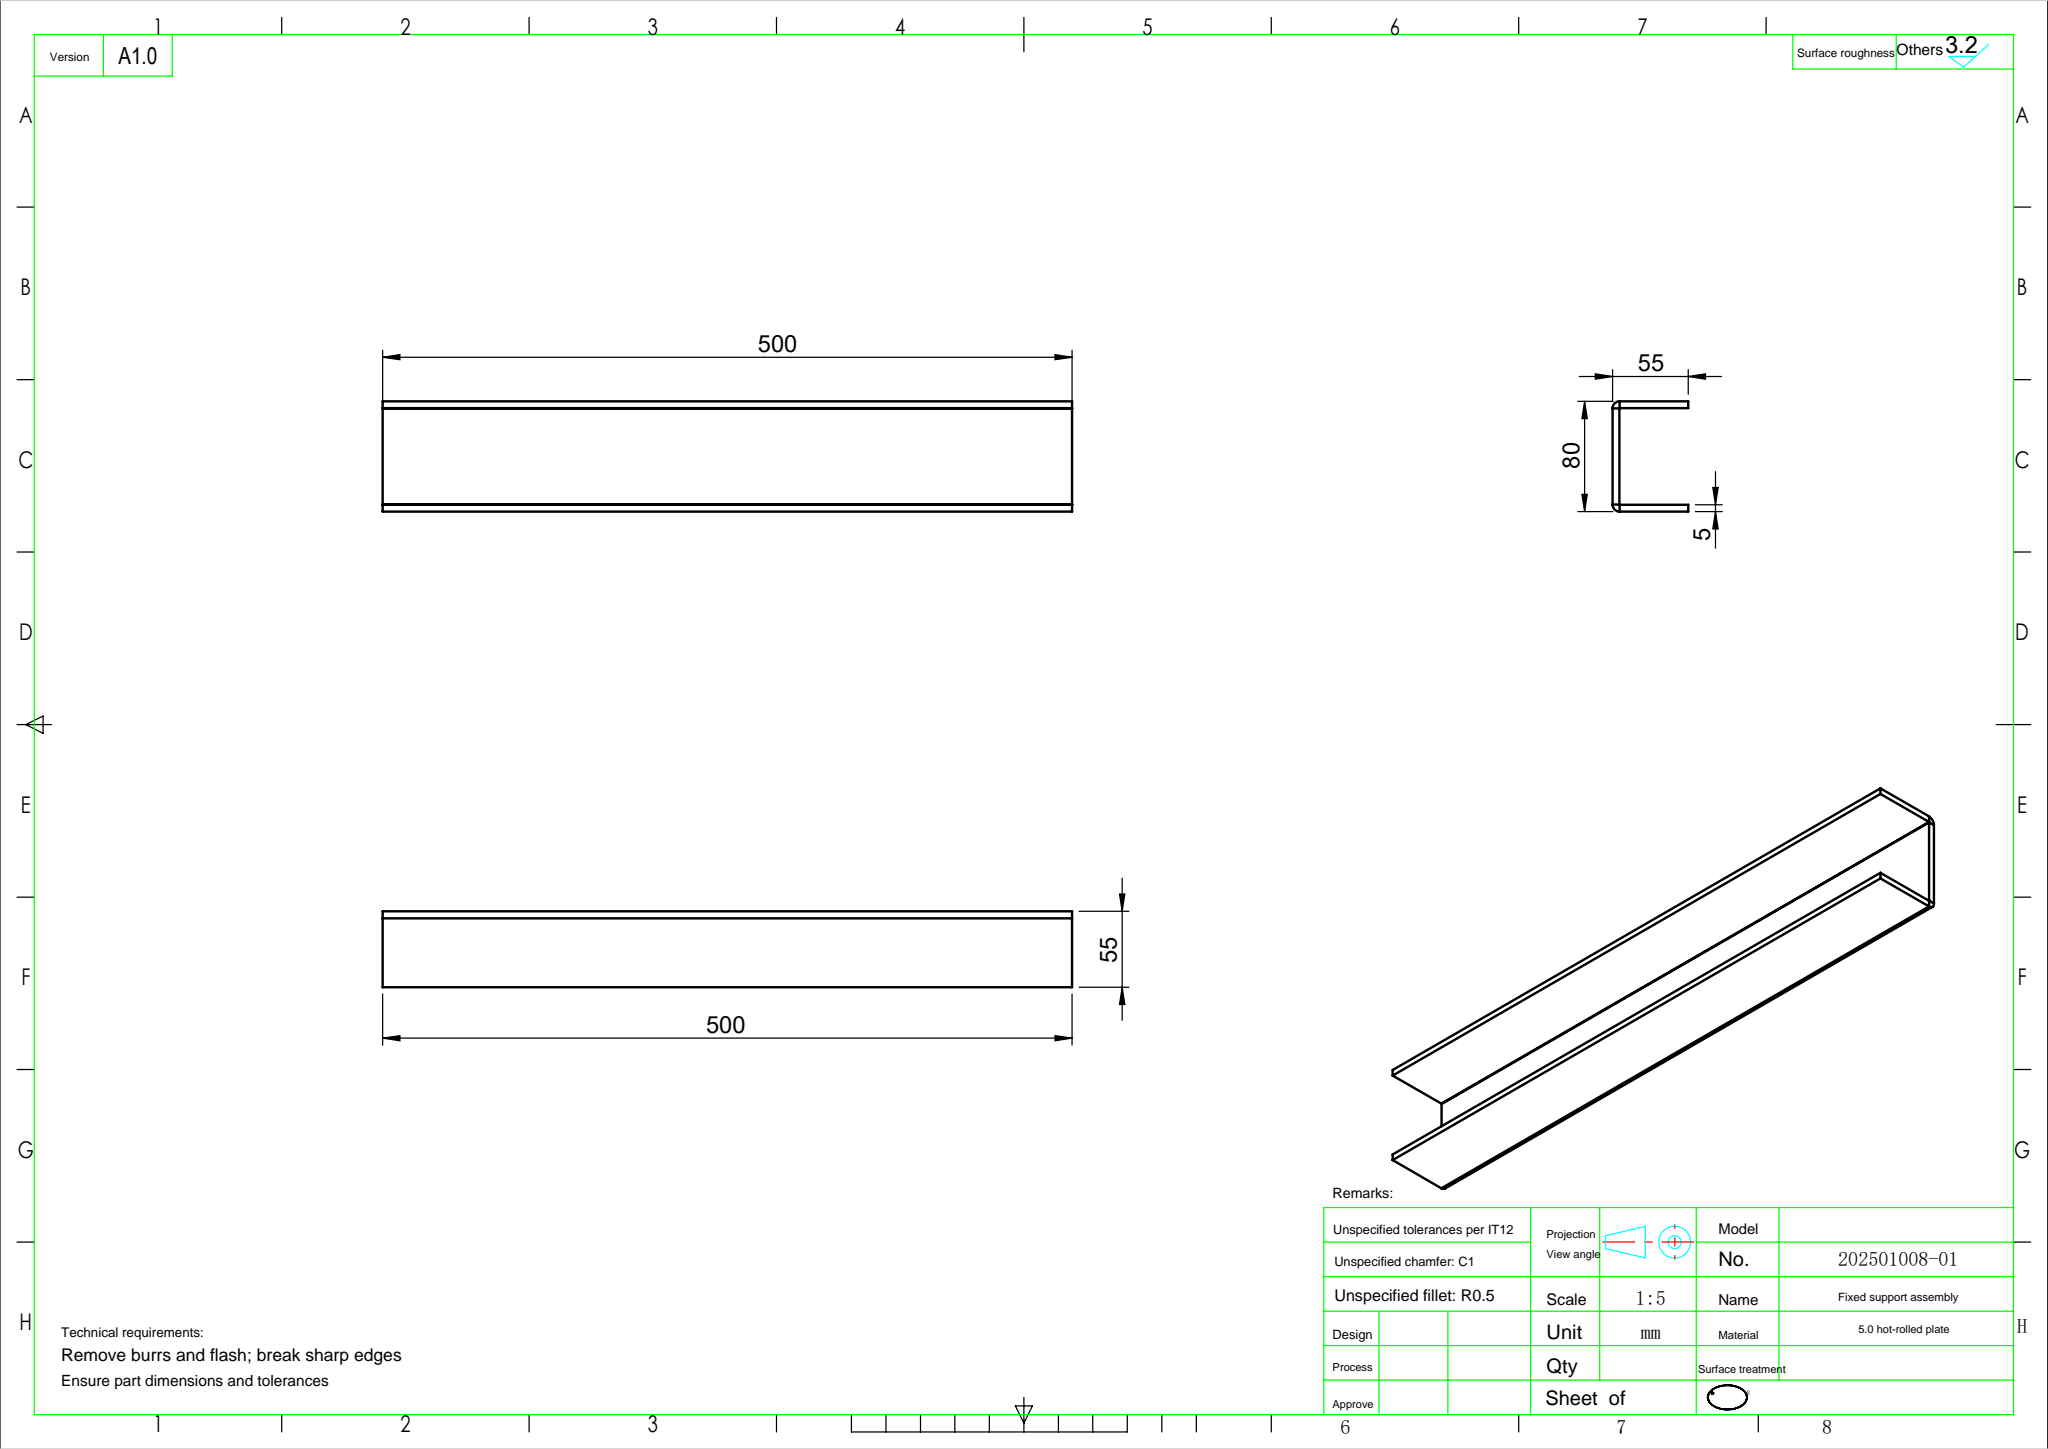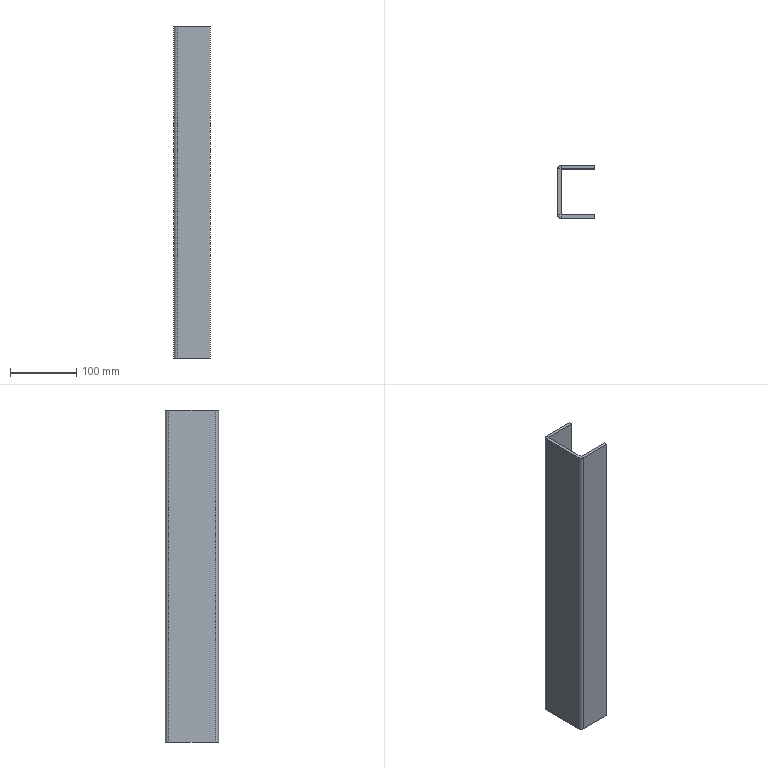Part | SolidWorks | features FlatPattern 1, SMBaseFlange 1, SheetMetal 1 | 1 solid | 22 faces | box 55 x 80 x 500 mm | volume 444206 mm3 | plane 18 | cylinder 4 | commonest cylinder face diameters 0.4 x2 10.4 x2
STEP:
#1=CARTESIAN_POINT('',(0.,34.8,500.));
#2=VERTEX_POINT('',#1);
#3=CARTESIAN_POINT('',(-5.,34.8,500.));
#4=VERTEX_POINT('',#3);
#5=CARTESIAN_POINT('',(0.,34.8,500.));
#6=DIRECTION('',(-1.,0.,0.));
#7=VECTOR('',#6,1000.);
#8=LINE('',#5,#7);
#9=EDGE_CURVE('',#2,#4,#8,.T.);
#10=ORIENTED_EDGE('',*,*,#9,.F.);
#11=CARTESIAN_POINT('',(0.2,35.,500.));
#12=VERTEX_POINT('',#11);
#13=CARTESIAN_POINT('',(0.2,34.8,500.));
#14=DIRECTION('',(0.,0.,1.));
#15=DIRECTION('',(-1.,0.,0.));
#16=AXIS2_PLACEMENT_3D('',#13,#14,#15);
#17=CIRCLE('',#16,0.2);
#18=EDGE_CURVE('',#12,#2,#17,.T.);
#19=ORIENTED_EDGE('',*,*,#18,.F.);
#20=CARTESIAN_POINT('',(0.2,40.,500.));
#21=VERTEX_POINT('',#20);
#22=CARTESIAN_POINT('',(0.2,40.,500.));
#23=DIRECTION('',(0.,-1.,0.));
#24=VECTOR('',#23,1000.);
#25=LINE('',#22,#24);
#26=EDGE_CURVE('',#21,#12,#25,.T.);
#27=ORIENTED_EDGE('',*,*,#26,.F.);
#28=CARTESIAN_POINT('',(0.2,34.8,500.));
#29=DIRECTION('',(0.,0.,1.));
#30=DIRECTION('',(1.,0.,0.));
#31=AXIS2_PLACEMENT_3D('',#28,#29,#30);
#32=CIRCLE('',#31,5.2);
#33=EDGE_CURVE('',#21,#4,#32,.T.);
#34=ORIENTED_EDGE('',*,*,#33,.T.);
#35=EDGE_LOOP('',(#10,#19,#27,#34));
#36=FACE_OUTER_BOUND('',#35,.T.);
#37=CARTESIAN_POINT('',(0.,34.8,500.));
#38=DIRECTION('',(0.,0.,1.));
#39=DIRECTION('',(1.,0.,0.));
#40=AXIS2_PLACEMENT_3D('',#37,#38,#39);
#41=PLANE('',#40);
#42=ADVANCED_FACE('',(#36),#41,.T.);
#43=CARTESIAN_POINT('',(0.,-34.8,500.));
#44=VERTEX_POINT('',#43);
#45=CARTESIAN_POINT('',(0.,35.,500.));
#46=DIRECTION('',(0.,-1.,0.));
#47=VECTOR('',#46,1000.);
#48=LINE('',#45,#47);
#49=EDGE_CURVE('',#2,#44,#48,.T.);
#50=ORIENTED_EDGE('',*,*,#49,.F.);
#51=ORIENTED_EDGE('',*,*,#9,.T.);
#52=CARTESIAN_POINT('',(-5.,-34.8,500.));
#53=VERTEX_POINT('',#52);
#54=CARTESIAN_POINT('',(-5.,35.,500.));
#55=DIRECTION('',(0.,-1.,0.));
#56=VECTOR('',#55,1000.);
#57=LINE('',#54,#56);
#58=EDGE_CURVE('',#4,#53,#57,.T.);
#59=ORIENTED_EDGE('',*,*,#58,.T.);
#60=CARTESIAN_POINT('',(-5.,-34.8,500.));
#61=DIRECTION('',(1.,0.,0.));
#62=VECTOR('',#61,1000.);
#63=LINE('',#60,#62);
#64=EDGE_CURVE('',#53,#44,#63,.T.);
#65=ORIENTED_EDGE('',*,*,#64,.T.);
#66=EDGE_LOOP('',(#50,#51,#59,#65));
#67=FACE_OUTER_BOUND('',#66,.T.);
#68=CARTESIAN_POINT('',(0.2,40.,500.));
#69=DIRECTION('',(0.,0.,1.));
#70=DIRECTION('',(1.,0.,0.));
#71=AXIS2_PLACEMENT_3D('',#68,#69,#70);
#72=PLANE('',#71);
#73=ADVANCED_FACE('',(#67),#72,.T.);
#74=CARTESIAN_POINT('',(0.2,35.,0.));
#75=VERTEX_POINT('',#74);
#76=CARTESIAN_POINT('',(0.2,40.,0.));
#77=VERTEX_POINT('',#76);
#78=CARTESIAN_POINT('',(0.2,35.,0.));
#79=DIRECTION('',(0.,1.,0.));
#80=VECTOR('',#79,1000.);
#81=LINE('',#78,#80);
#82=EDGE_CURVE('',#75,#77,#81,.T.);
#83=ORIENTED_EDGE('',*,*,#82,.F.);
#84=CARTESIAN_POINT('',(0.,34.8,0.));
#85=VERTEX_POINT('',#84);
#86=CARTESIAN_POINT('',(0.2,34.8,0.));
#87=DIRECTION('',(0.,0.,1.));
#88=DIRECTION('',(-1.,0.,0.));
#89=AXIS2_PLACEMENT_3D('',#86,#87,#88);
#90=CIRCLE('',#89,0.2);
#91=EDGE_CURVE('',#75,#85,#90,.T.);
#92=ORIENTED_EDGE('',*,*,#91,.T.);
#93=CARTESIAN_POINT('',(-5.,34.8,0.));
#94=VERTEX_POINT('',#93);
#95=CARTESIAN_POINT('',(-5.,34.8,0.));
#96=DIRECTION('',(1.,0.,0.));
#97=VECTOR('',#96,1000.);
#98=LINE('',#95,#97);
#99=EDGE_CURVE('',#94,#85,#98,.T.);
#100=ORIENTED_EDGE('',*,*,#99,.F.);
#101=CARTESIAN_POINT('',(0.2,34.8,0.));
#102=DIRECTION('',(0.,0.,1.));
#103=DIRECTION('',(1.,0.,0.));
#104=AXIS2_PLACEMENT_3D('',#101,#102,#103);
#105=CIRCLE('',#104,5.2);
#106=EDGE_CURVE('',#77,#94,#105,.T.);
#107=ORIENTED_EDGE('',*,*,#106,.F.);
#108=EDGE_LOOP('',(#83,#92,#100,#107));
#109=FACE_OUTER_BOUND('',#108,.T.);
#110=CARTESIAN_POINT('',(0.2,35.,0.));
#111=DIRECTION('',(0.,0.,-1.));
#112=DIRECTION('',(-1.,0.,0.));
#113=AXIS2_PLACEMENT_3D('',#110,#111,#112);
#114=PLANE('',#113);
#115=ADVANCED_FACE('',(#109),#114,.T.);
#116=CARTESIAN_POINT('',(50.,35.,0.));
#117=VERTEX_POINT('',#116);
#118=CARTESIAN_POINT('',(0.,35.,0.));
#119=DIRECTION('',(-1.,0.,0.));
#120=VECTOR('',#119,1000.);
#121=LINE('',#118,#120);
#122=EDGE_CURVE('',#117,#75,#121,.T.);
#123=ORIENTED_EDGE('',*,*,#122,.T.);
#124=ORIENTED_EDGE('',*,*,#82,.T.);
#125=CARTESIAN_POINT('',(50.,40.,0.));
#126=VERTEX_POINT('',#125);
#127=CARTESIAN_POINT('',(0.,40.,0.));
#128=DIRECTION('',(-1.,0.,0.));
#129=VECTOR('',#128,1000.);
#130=LINE('',#127,#129);
#131=EDGE_CURVE('',#126,#77,#130,.T.);
#132=ORIENTED_EDGE('',*,*,#131,.F.);
#133=CARTESIAN_POINT('',(50.,40.,0.));
#134=DIRECTION('',(0.,-1.,0.));
#135=VECTOR('',#134,1000.);
#136=LINE('',#133,#135);
#137=EDGE_CURVE('',#126,#117,#136,.T.);
#138=ORIENTED_EDGE('',*,*,#137,.T.);
#139=EDGE_LOOP('',(#123,#124,#132,#138));
#140=FACE_OUTER_BOUND('',#139,.T.);
#141=CARTESIAN_POINT('',(-5.,34.8,0.));
#142=DIRECTION('',(0.,0.,-1.));
#143=DIRECTION('',(-1.,0.,0.));
#144=AXIS2_PLACEMENT_3D('',#141,#142,#143);
#145=PLANE('',#144);
#146=ADVANCED_FACE('',(#140),#145,.T.);
#147=CARTESIAN_POINT('',(0.2,-35.,500.));
#148=VERTEX_POINT('',#147);
#149=CARTESIAN_POINT('',(0.2,-40.,500.));
#150=VERTEX_POINT('',#149);
#151=CARTESIAN_POINT('',(0.2,-35.,500.));
#152=DIRECTION('',(0.,-1.,0.));
#153=VECTOR('',#152,1000.);
#154=LINE('',#151,#153);
#155=EDGE_CURVE('',#148,#150,#154,.T.);
#156=ORIENTED_EDGE('',*,*,#155,.F.);
#157=CARTESIAN_POINT('',(0.2,-34.8,500.));
#158=DIRECTION('',(0.,0.,1.));
#159=DIRECTION('',(-1.,0.,0.));
#160=AXIS2_PLACEMENT_3D('',#157,#158,#159);
#161=CIRCLE('',#160,0.2);
#162=EDGE_CURVE('',#44,#148,#161,.T.);
#163=ORIENTED_EDGE('',*,*,#162,.F.);
#164=ORIENTED_EDGE('',*,*,#64,.F.);
#165=CARTESIAN_POINT('',(0.2,-34.8,500.));
#166=DIRECTION('',(0.,0.,1.));
#167=DIRECTION('',(1.,0.,0.));
#168=AXIS2_PLACEMENT_3D('',#165,#166,#167);
#169=CIRCLE('',#168,5.2);
#170=EDGE_CURVE('',#53,#150,#169,.T.);
#171=ORIENTED_EDGE('',*,*,#170,.T.);
#172=EDGE_LOOP('',(#156,#163,#164,#171));
#173=FACE_OUTER_BOUND('',#172,.T.);
#174=CARTESIAN_POINT('',(0.2,-35.,500.));
#175=DIRECTION('',(0.,0.,1.));
#176=DIRECTION('',(1.,0.,0.));
#177=AXIS2_PLACEMENT_3D('',#174,#175,#176);
#178=PLANE('',#177);
#179=ADVANCED_FACE('',(#173),#178,.T.);
#180=CARTESIAN_POINT('',(50.,-35.,500.));
#181=VERTEX_POINT('',#180);
#182=CARTESIAN_POINT('',(0.,-35.,500.));
#183=DIRECTION('',(1.,0.,0.));
#184=VECTOR('',#183,1000.);
#185=LINE('',#182,#184);
#186=EDGE_CURVE('',#148,#181,#185,.T.);
#187=ORIENTED_EDGE('',*,*,#186,.F.);
#188=ORIENTED_EDGE('',*,*,#155,.T.);
#189=CARTESIAN_POINT('',(50.,-40.,500.));
#190=VERTEX_POINT('',#189);
#191=CARTESIAN_POINT('',(0.,-40.,500.));
#192=DIRECTION('',(1.,0.,0.));
#193=VECTOR('',#192,1000.);
#194=LINE('',#191,#193);
#195=EDGE_CURVE('',#150,#190,#194,.T.);
#196=ORIENTED_EDGE('',*,*,#195,.T.);
#197=CARTESIAN_POINT('',(50.,-35.,500.));
#198=DIRECTION('',(0.,-1.,0.));
#199=VECTOR('',#198,1000.);
#200=LINE('',#197,#199);
#201=EDGE_CURVE('',#181,#190,#200,.T.);
#202=ORIENTED_EDGE('',*,*,#201,.F.);
#203=EDGE_LOOP('',(#187,#188,#196,#202));
#204=FACE_OUTER_BOUND('',#203,.T.);
#205=CARTESIAN_POINT('',(-5.,-34.8,500.));
#206=DIRECTION('',(0.,0.,1.));
#207=DIRECTION('',(1.,0.,0.));
#208=AXIS2_PLACEMENT_3D('',#205,#206,#207);
#209=PLANE('',#208);
#210=ADVANCED_FACE('',(#204),#209,.T.);
#211=CARTESIAN_POINT('',(0.,-34.8,0.));
#212=VERTEX_POINT('',#211);
#213=CARTESIAN_POINT('',(-5.,-34.8,0.));
#214=VERTEX_POINT('',#213);
#215=CARTESIAN_POINT('',(0.,-34.8,0.));
#216=DIRECTION('',(-1.,0.,0.));
#217=VECTOR('',#216,1000.);
#218=LINE('',#215,#217);
#219=EDGE_CURVE('',#212,#214,#218,.T.);
#220=ORIENTED_EDGE('',*,*,#219,.F.);
#221=CARTESIAN_POINT('',(0.2,-35.,0.));
#222=VERTEX_POINT('',#221);
#223=CARTESIAN_POINT('',(0.2,-34.8,0.));
#224=DIRECTION('',(0.,0.,1.));
#225=DIRECTION('',(-1.,0.,0.));
#226=AXIS2_PLACEMENT_3D('',#223,#224,#225);
#227=CIRCLE('',#226,0.2);
#228=EDGE_CURVE('',#212,#222,#227,.T.);
#229=ORIENTED_EDGE('',*,*,#228,.T.);
#230=CARTESIAN_POINT('',(0.2,-40.,0.));
#231=VERTEX_POINT('',#230);
#232=CARTESIAN_POINT('',(0.2,-40.,0.));
#233=DIRECTION('',(0.,1.,0.));
#234=VECTOR('',#233,1000.);
#235=LINE('',#232,#234);
#236=EDGE_CURVE('',#231,#222,#235,.T.);
#237=ORIENTED_EDGE('',*,*,#236,.F.);
#238=CARTESIAN_POINT('',(0.2,-34.8,0.));
#239=DIRECTION('',(0.,0.,1.));
#240=DIRECTION('',(1.,0.,0.));
#241=AXIS2_PLACEMENT_3D('',#238,#239,#240);
#242=CIRCLE('',#241,5.2);
#243=EDGE_CURVE('',#214,#231,#242,.T.);
#244=ORIENTED_EDGE('',*,*,#243,.F.);
#245=EDGE_LOOP('',(#220,#229,#237,#244));
#246=FACE_OUTER_BOUND('',#245,.T.);
#247=CARTESIAN_POINT('',(0.,-34.8,0.));
#248=DIRECTION('',(0.,0.,-1.));
#249=DIRECTION('',(-1.,0.,0.));
#250=AXIS2_PLACEMENT_3D('',#247,#248,#249);
#251=PLANE('',#250);
#252=ADVANCED_FACE('',(#246),#251,.T.);
#253=CARTESIAN_POINT('',(0.,35.,0.));
#254=DIRECTION('',(0.,-1.,0.));
#255=VECTOR('',#254,1000.);
#256=LINE('',#253,#255);
#257=EDGE_CURVE('',#85,#212,#256,.T.);
#258=ORIENTED_EDGE('',*,*,#257,.T.);
#259=ORIENTED_EDGE('',*,*,#219,.T.);
#260=CARTESIAN_POINT('',(-5.,35.,0.));
#261=DIRECTION('',(0.,-1.,0.));
#262=VECTOR('',#261,1000.);
#263=LINE('',#260,#262);
#264=EDGE_CURVE('',#94,#214,#263,.T.);
#265=ORIENTED_EDGE('',*,*,#264,.F.);
#266=ORIENTED_EDGE('',*,*,#99,.T.);
#267=EDGE_LOOP('',(#258,#259,#265,#266));
#268=FACE_OUTER_BOUND('',#267,.T.);
#269=CARTESIAN_POINT('',(0.2,-40.,0.));
#270=DIRECTION('',(0.,0.,-1.));
#271=DIRECTION('',(-1.,0.,0.));
#272=AXIS2_PLACEMENT_3D('',#269,#270,#271);
#273=PLANE('',#272);
#274=ADVANCED_FACE('',(#268),#273,.T.);
#275=CARTESIAN_POINT('',(50.,-40.,0.));
#276=VERTEX_POINT('',#275);
#277=CARTESIAN_POINT('',(0.,-40.,0.));
#278=DIRECTION('',(1.,0.,0.));
#279=VECTOR('',#278,1000.);
#280=LINE('',#277,#279);
#281=EDGE_CURVE('',#231,#276,#280,.T.);
#282=ORIENTED_EDGE('',*,*,#281,.T.);
#283=CARTESIAN_POINT('',(50.,-40.,500.));
#284=DIRECTION('',(0.,0.,-1.));
#285=VECTOR('',#284,1000.);
#286=LINE('',#283,#285);
#287=EDGE_CURVE('',#190,#276,#286,.T.);
#288=ORIENTED_EDGE('',*,*,#287,.F.);
#289=ORIENTED_EDGE('',*,*,#195,.F.);
#290=CARTESIAN_POINT('',(0.2,-40.,500.));
#291=DIRECTION('',(0.,0.,-1.));
#292=VECTOR('',#291,1000.);
#293=LINE('',#290,#292);
#294=EDGE_CURVE('',#150,#231,#293,.T.);
#295=ORIENTED_EDGE('',*,*,#294,.T.);
#296=EDGE_LOOP('',(#282,#288,#289,#295));
#297=FACE_OUTER_BOUND('',#296,.T.);
#298=CARTESIAN_POINT('',(0.,-40.,500.));
#299=DIRECTION('',(0.,1.,0.));
#300=DIRECTION('',(0.,0.,1.));
#301=AXIS2_PLACEMENT_3D('',#298,#299,#300);
#302=PLANE('',#301);
#303=ADVANCED_FACE('',(#297),#302,.F.);
#304=CARTESIAN_POINT('',(50.,-35.,0.));
#305=VERTEX_POINT('',#304);
#306=CARTESIAN_POINT('',(50.,-35.,0.));
#307=DIRECTION('',(0.,-1.,0.));
#308=VECTOR('',#307,1000.);
#309=LINE('',#306,#308);
#310=EDGE_CURVE('',#305,#276,#309,.T.);
#311=ORIENTED_EDGE('',*,*,#310,.F.);
#312=CARTESIAN_POINT('',(50.,-35.,500.));
#313=DIRECTION('',(0.,0.,-1.));
#314=VECTOR('',#313,1000.);
#315=LINE('',#312,#314);
#316=EDGE_CURVE('',#181,#305,#315,.T.);
#317=ORIENTED_EDGE('',*,*,#316,.F.);
#318=ORIENTED_EDGE('',*,*,#201,.T.);
#319=ORIENTED_EDGE('',*,*,#287,.T.);
#320=EDGE_LOOP('',(#311,#317,#318,#319));
#321=FACE_OUTER_BOUND('',#320,.T.);
#322=CARTESIAN_POINT('',(50.,-35.,500.));
#323=DIRECTION('',(1.,0.,0.));
#324=DIRECTION('',(0.,0.,-1.));
#325=AXIS2_PLACEMENT_3D('',#322,#323,#324);
#326=PLANE('',#325);
#327=ADVANCED_FACE('',(#321),#326,.T.);
#328=CARTESIAN_POINT('',(0.,-35.,0.));
#329=DIRECTION('',(1.,0.,0.));
#330=VECTOR('',#329,1000.);
#331=LINE('',#328,#330);
#332=EDGE_CURVE('',#222,#305,#331,.T.);
#333=ORIENTED_EDGE('',*,*,#332,.F.);
#334=CARTESIAN_POINT('',(0.2,-35.,500.));
#335=DIRECTION('',(0.,0.,-1.));
#336=VECTOR('',#335,1000.);
#337=LINE('',#334,#336);
#338=EDGE_CURVE('',#148,#222,#337,.T.);
#339=ORIENTED_EDGE('',*,*,#338,.F.);
#340=ORIENTED_EDGE('',*,*,#186,.T.);
#341=ORIENTED_EDGE('',*,*,#316,.T.);
#342=EDGE_LOOP('',(#333,#339,#340,#341));
#343=FACE_OUTER_BOUND('',#342,.T.);
#344=CARTESIAN_POINT('',(0.,-35.,500.));
#345=DIRECTION('',(0.,1.,0.));
#346=DIRECTION('',(0.,0.,1.));
#347=AXIS2_PLACEMENT_3D('',#344,#345,#346);
#348=PLANE('',#347);
#349=ADVANCED_FACE('',(#343),#348,.T.);
#350=ORIENTED_EDGE('',*,*,#228,.F.);
#351=CARTESIAN_POINT('',(0.,-34.8,500.));
#352=DIRECTION('',(0.,0.,-1.));
#353=VECTOR('',#352,1000.);
#354=LINE('',#351,#353);
#355=EDGE_CURVE('',#44,#212,#354,.T.);
#356=ORIENTED_EDGE('',*,*,#355,.F.);
#357=ORIENTED_EDGE('',*,*,#162,.T.);
#358=ORIENTED_EDGE('',*,*,#338,.T.);
#359=EDGE_LOOP('',(#350,#356,#357,#358));
#360=FACE_OUTER_BOUND('',#359,.T.);
#361=CARTESIAN_POINT('',(0.2,-34.8,500.));
#362=DIRECTION('',(0.,0.,-1.));
#363=DIRECTION('',(-1.,0.,0.));
#364=AXIS2_PLACEMENT_3D('',#361,#362,#363);
#365=CYLINDRICAL_SURFACE('',#364,0.2);
#366=ADVANCED_FACE('',(#360),#365,.F.);
#367=ORIENTED_EDGE('',*,*,#257,.F.);
#368=CARTESIAN_POINT('',(0.,34.8,500.));
#369=DIRECTION('',(0.,0.,-1.));
#370=VECTOR('',#369,1000.);
#371=LINE('',#368,#370);
#372=EDGE_CURVE('',#2,#85,#371,.T.);
#373=ORIENTED_EDGE('',*,*,#372,.F.);
#374=ORIENTED_EDGE('',*,*,#49,.T.);
#375=ORIENTED_EDGE('',*,*,#355,.T.);
#376=EDGE_LOOP('',(#367,#373,#374,#375));
#377=FACE_OUTER_BOUND('',#376,.T.);
#378=CARTESIAN_POINT('',(0.,35.,500.));
#379=DIRECTION('',(1.,0.,0.));
#380=DIRECTION('',(0.,0.,-1.));
#381=AXIS2_PLACEMENT_3D('',#378,#379,#380);
#382=PLANE('',#381);
#383=ADVANCED_FACE('',(#377),#382,.T.);
#384=ORIENTED_EDGE('',*,*,#91,.F.);
#385=CARTESIAN_POINT('',(0.2,35.,500.));
#386=DIRECTION('',(0.,0.,-1.));
#387=VECTOR('',#386,1000.);
#388=LINE('',#385,#387);
#389=EDGE_CURVE('',#12,#75,#388,.T.);
#390=ORIENTED_EDGE('',*,*,#389,.F.);
#391=ORIENTED_EDGE('',*,*,#18,.T.);
#392=ORIENTED_EDGE('',*,*,#372,.T.);
#393=EDGE_LOOP('',(#384,#390,#391,#392));
#394=FACE_OUTER_BOUND('',#393,.T.);
#395=CARTESIAN_POINT('',(0.2,34.8,500.));
#396=DIRECTION('',(0.,0.,-1.));
#397=DIRECTION('',(-1.,0.,0.));
#398=AXIS2_PLACEMENT_3D('',#395,#396,#397);
#399=CYLINDRICAL_SURFACE('',#398,0.2);
#400=ADVANCED_FACE('',(#394),#399,.F.);
#401=ORIENTED_EDGE('',*,*,#122,.F.);
#402=CARTESIAN_POINT('',(50.,35.,500.));
#403=VERTEX_POINT('',#402);
#404=CARTESIAN_POINT('',(50.,35.,500.));
#405=DIRECTION('',(0.,0.,-1.));
#406=VECTOR('',#405,1000.);
#407=LINE('',#404,#406);
#408=EDGE_CURVE('',#403,#117,#407,.T.);
#409=ORIENTED_EDGE('',*,*,#408,.F.);
#410=CARTESIAN_POINT('',(0.,35.,500.));
#411=DIRECTION('',(-1.,0.,0.));
#412=VECTOR('',#411,1000.);
#413=LINE('',#410,#412);
#414=EDGE_CURVE('',#403,#12,#413,.T.);
#415=ORIENTED_EDGE('',*,*,#414,.T.);
#416=ORIENTED_EDGE('',*,*,#389,.T.);
#417=EDGE_LOOP('',(#401,#409,#415,#416));
#418=FACE_OUTER_BOUND('',#417,.T.);
#419=CARTESIAN_POINT('',(0.,35.,500.));
#420=DIRECTION('',(0.,-1.,0.));
#421=DIRECTION('',(0.,0.,-1.));
#422=AXIS2_PLACEMENT_3D('',#419,#420,#421);
#423=PLANE('',#422);
#424=ADVANCED_FACE('',(#418),#423,.T.);
#425=ORIENTED_EDGE('',*,*,#137,.F.);
#426=CARTESIAN_POINT('',(50.,40.,500.));
#427=VERTEX_POINT('',#426);
#428=CARTESIAN_POINT('',(50.,40.,500.));
#429=DIRECTION('',(0.,0.,-1.));
#430=VECTOR('',#429,1000.);
#431=LINE('',#428,#430);
#432=EDGE_CURVE('',#427,#126,#431,.T.);
#433=ORIENTED_EDGE('',*,*,#432,.F.);
#434=CARTESIAN_POINT('',(50.,40.,500.));
#435=DIRECTION('',(0.,-1.,0.));
#436=VECTOR('',#435,1000.);
#437=LINE('',#434,#436);
#438=EDGE_CURVE('',#427,#403,#437,.T.);
#439=ORIENTED_EDGE('',*,*,#438,.T.);
#440=ORIENTED_EDGE('',*,*,#408,.T.);
#441=EDGE_LOOP('',(#425,#433,#439,#440));
#442=FACE_OUTER_BOUND('',#441,.T.);
#443=CARTESIAN_POINT('',(50.,40.,500.));
#444=DIRECTION('',(1.,0.,0.));
#445=DIRECTION('',(0.,0.,-1.));
#446=AXIS2_PLACEMENT_3D('',#443,#444,#445);
#447=PLANE('',#446);
#448=ADVANCED_FACE('',(#442),#447,.T.);
#449=ORIENTED_EDGE('',*,*,#131,.T.);
#450=CARTESIAN_POINT('',(0.2,40.,500.));
#451=DIRECTION('',(0.,0.,-1.));
#452=VECTOR('',#451,1000.);
#453=LINE('',#450,#452);
#454=EDGE_CURVE('',#21,#77,#453,.T.);
#455=ORIENTED_EDGE('',*,*,#454,.F.);
#456=CARTESIAN_POINT('',(0.,40.,500.));
#457=DIRECTION('',(-1.,0.,0.));
#458=VECTOR('',#457,1000.);
#459=LINE('',#456,#458);
#460=EDGE_CURVE('',#427,#21,#459,.T.);
#461=ORIENTED_EDGE('',*,*,#460,.F.);
#462=ORIENTED_EDGE('',*,*,#432,.T.);
#463=EDGE_LOOP('',(#449,#455,#461,#462));
#464=FACE_OUTER_BOUND('',#463,.T.);
#465=CARTESIAN_POINT('',(0.,40.,500.));
#466=DIRECTION('',(0.,-1.,0.));
#467=DIRECTION('',(0.,0.,-1.));
#468=AXIS2_PLACEMENT_3D('',#465,#466,#467);
#469=PLANE('',#468);
#470=ADVANCED_FACE('',(#464),#469,.F.);
#471=ORIENTED_EDGE('',*,*,#106,.T.);
#472=CARTESIAN_POINT('',(-5.,34.8,500.));
#473=DIRECTION('',(0.,0.,-1.));
#474=VECTOR('',#473,1000.);
#475=LINE('',#472,#474);
#476=EDGE_CURVE('',#4,#94,#475,.T.);
#477=ORIENTED_EDGE('',*,*,#476,.F.);
#478=ORIENTED_EDGE('',*,*,#33,.F.);
#479=ORIENTED_EDGE('',*,*,#454,.T.);
#480=EDGE_LOOP('',(#471,#477,#478,#479));
#481=FACE_OUTER_BOUND('',#480,.T.);
#482=CARTESIAN_POINT('',(0.2,34.8,500.));
#483=DIRECTION('',(0.,0.,-1.));
#484=DIRECTION('',(-1.,0.,0.));
#485=AXIS2_PLACEMENT_3D('',#482,#483,#484);
#486=CYLINDRICAL_SURFACE('',#485,5.2);
#487=ADVANCED_FACE('',(#481),#486,.T.);
#488=ORIENTED_EDGE('',*,*,#264,.T.);
#489=CARTESIAN_POINT('',(-5.,-34.8,500.));
#490=DIRECTION('',(0.,0.,-1.));
#491=VECTOR('',#490,1000.);
#492=LINE('',#489,#491);
#493=EDGE_CURVE('',#53,#214,#492,.T.);
#494=ORIENTED_EDGE('',*,*,#493,.F.);
#495=ORIENTED_EDGE('',*,*,#58,.F.);
#496=ORIENTED_EDGE('',*,*,#476,.T.);
#497=EDGE_LOOP('',(#488,#494,#495,#496));
#498=FACE_OUTER_BOUND('',#497,.T.);
#499=CARTESIAN_POINT('',(-5.,35.,500.));
#500=DIRECTION('',(1.,0.,0.));
#501=DIRECTION('',(0.,0.,-1.));
#502=AXIS2_PLACEMENT_3D('',#499,#500,#501);
#503=PLANE('',#502);
#504=ADVANCED_FACE('',(#498),#503,.F.);
#505=ORIENTED_EDGE('',*,*,#243,.T.);
#506=ORIENTED_EDGE('',*,*,#294,.F.);
#507=ORIENTED_EDGE('',*,*,#170,.F.);
#508=ORIENTED_EDGE('',*,*,#493,.T.);
#509=EDGE_LOOP('',(#505,#506,#507,#508));
#510=FACE_OUTER_BOUND('',#509,.T.);
#511=CARTESIAN_POINT('',(0.2,-34.8,500.));
#512=DIRECTION('',(0.,0.,-1.));
#513=DIRECTION('',(-1.,0.,0.));
#514=AXIS2_PLACEMENT_3D('',#511,#512,#513);
#515=CYLINDRICAL_SURFACE('',#514,5.2);
#516=ADVANCED_FACE('',(#510),#515,.T.);
#517=ORIENTED_EDGE('',*,*,#460,.T.);
#518=ORIENTED_EDGE('',*,*,#26,.T.);
#519=ORIENTED_EDGE('',*,*,#414,.F.);
#520=ORIENTED_EDGE('',*,*,#438,.F.);
#521=EDGE_LOOP('',(#517,#518,#519,#520));
#522=FACE_OUTER_BOUND('',#521,.T.);
#523=CARTESIAN_POINT('',(0.2,-34.8,500.));
#524=DIRECTION('',(0.,0.,-1.));
#525=DIRECTION('',(-1.,0.,0.));
#526=AXIS2_PLACEMENT_3D('',#523,#524,#525);
#527=PLANE('',#526);
#528=ADVANCED_FACE('',(#522),#527,.F.);
#529=ORIENTED_EDGE('',*,*,#281,.F.);
#530=ORIENTED_EDGE('',*,*,#236,.T.);
#531=ORIENTED_EDGE('',*,*,#332,.T.);
#532=ORIENTED_EDGE('',*,*,#310,.T.);
#533=EDGE_LOOP('',(#529,#530,#531,#532));
#534=FACE_OUTER_BOUND('',#533,.T.);
#535=CARTESIAN_POINT('',(0.2,-34.8,0.));
#536=DIRECTION('',(0.,0.,-1.));
#537=DIRECTION('',(-1.,0.,0.));
#538=AXIS2_PLACEMENT_3D('',#535,#536,#537);
#539=PLANE('',#538);
#540=ADVANCED_FACE('',(#534),#539,.T.);
#541=CLOSED_SHELL('',(#42,#73,#115,#146,#179,#210,#252,#274,#303,#327,#349,#366,#383,#400,#424,#448,#470,#487,#504,#516,#528,#540));
#542=MANIFOLD_SOLID_BREP('',#541);
#543=CARTESIAN_POINT('',(0.,0.,0.));
#544=DIRECTION('',(0.,0.,1.));
#545=DIRECTION('',(1.,0.,0.));
#546=AXIS2_PLACEMENT_3D('',#543,#544,#545);
#547=(LENGTH_UNIT()NAMED_UNIT(*)SI_UNIT(.MILLI.,.METRE.));
#548=UNCERTAINTY_MEASURE_WITH_UNIT(LENGTH_MEASURE(0.00001),#547,'','');
#549=(NAMED_UNIT(*)PLANE_ANGLE_UNIT()SI_UNIT($,.RADIAN.));
#550=(NAMED_UNIT(*)SI_UNIT($,.STERADIAN.)SOLID_ANGLE_UNIT());
#551=(GEOMETRIC_REPRESENTATION_CONTEXT(3)GLOBAL_UNCERTAINTY_ASSIGNED_CONTEXT((#548))GLOBAL_UNIT_ASSIGNED_CONTEXT((#547,#549,#550))REPRESENTATION_CONTEXT('',''));
#552=ADVANCED_BREP_SHAPE_REPRESENTATION('',(#542,#546),#551);